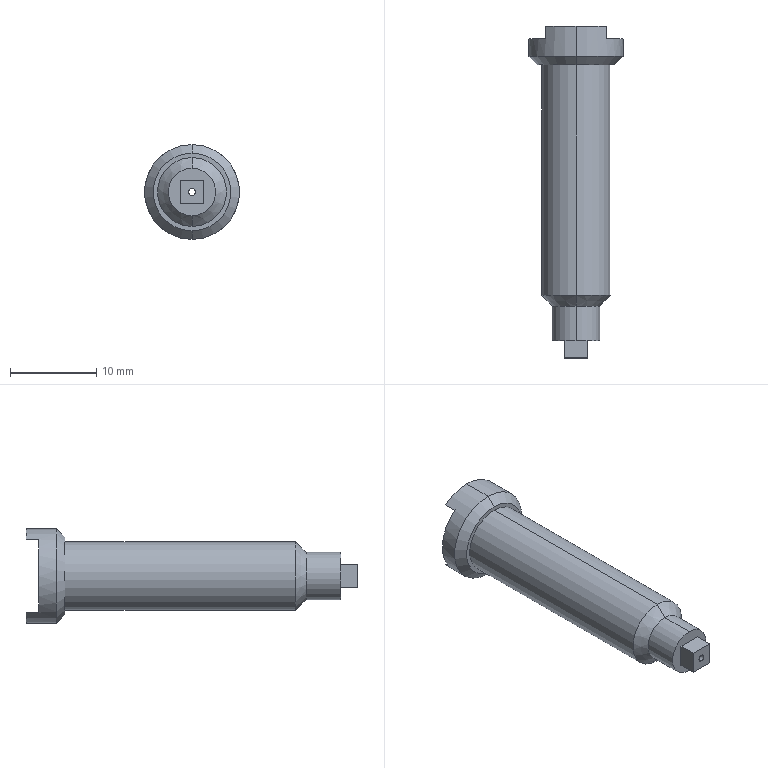Part | STEP file | 1 solid | 33 faces | box 11 x 38.5 x 11 mm | volume 1504 mm3 | plane 15 | cylinder 14 | cone 4 | commonest cylinder face diameters 8 x4 0.8 x2 1.5 x2 3 x2 5.5 x2 11 x2